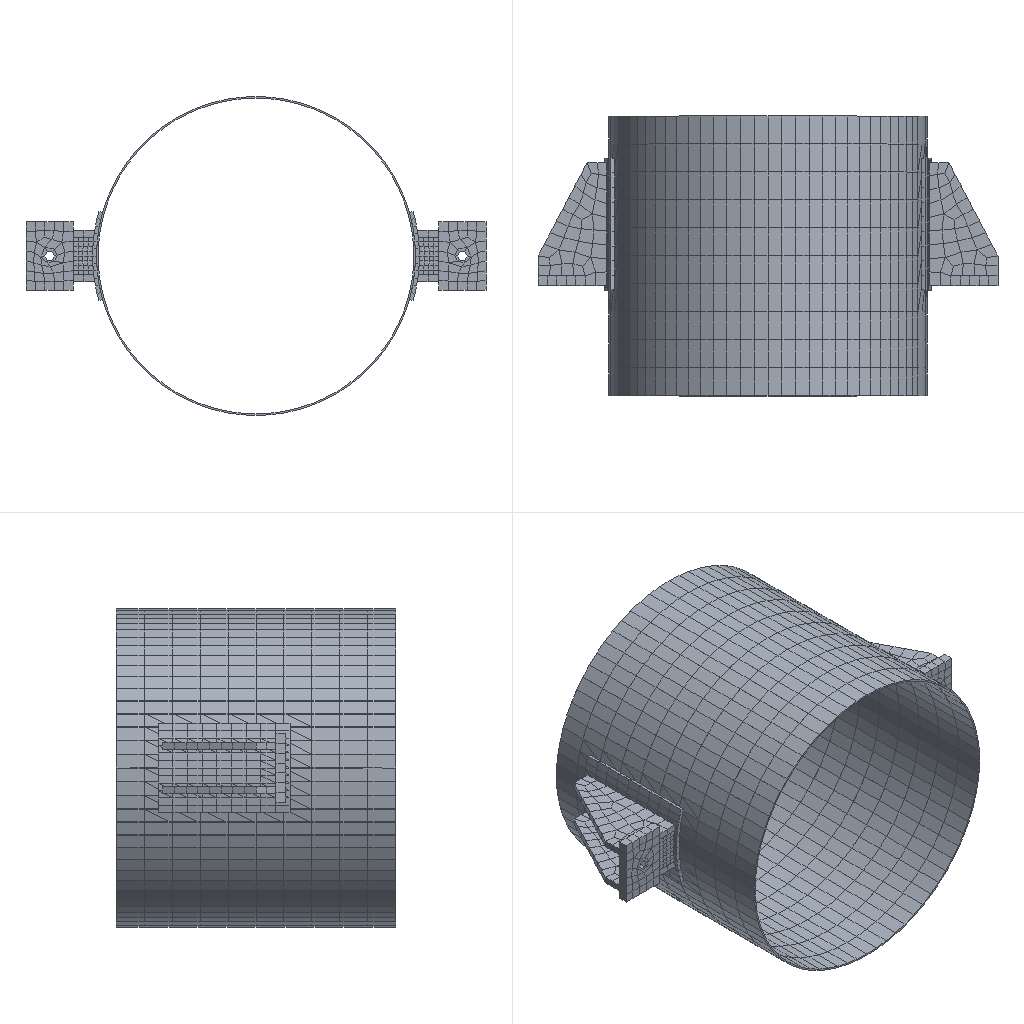Simulation study | ansys workbench
Ansys APDL input file, long lists of numbers shortened:
/batch
/config,noeldb,1     ! force off writing results to database
*get,_wallstrt,active,,time,wall
! ANSYS input file written by Workbench version 2022 R1
! File used for geometry attach:
/title,wbnew--____ (B5)
! ****** Begin Custom Load Command Snippet ******
/COM, ACT Extensions:
/COM,     LSDYNA, 2021.1
/COM,
! ****** End   Custom Load Command Snippet ******
*DIM,_wb_ProjectScratch_dir,string,248
_wb_ProjectScratch_dir(1) = ''
*DIM,_wb_SolverFiles_dir,string,248
_wb_SolverFiles_dir(1) = ''
*DIM,_wb_userfiles_dir,string,248
_wb_userfiles_dir(1) = ''
/com,--- Data in consistent NMM units. See Solving Units in the help system for more information.
/units,MPA
/nopr
/wb,file,start              !  signify a WB generated input file
/prep7
! Turn off shape checking because checks already performed inside WB mesher.
! See help system for more information.
SHPP,OFF,,NOWARN
/nolist
etcon,set             ! allow ANSYS to choose best KEYOP's for 180x elements, resets any applicable keyopt to MAPDL defaults
/com,*********** Nodes for the whole assembly ***********
nblock,3,,11156
(1i9,3e20.9e3)
        1    -9.929159159E+02     6.715040761E+02    -9.500000000E+01
! (10141 more lines like these left out)
-1
/wb,elem,start            !  set before creation of elements
/com,*********** Elements for Body 1 "__1^___1|__-__1" ***********
et,1,186
keyo,1,2,1          ! set full integration on SOLID186
eblock,19,solid,,720
(19i9)
        1        1        1        1        0        0        0        0       20        0      583     5200     5908     5907     5201     5204     5943     5942     5202
! (1439 more lines like these left out)
-1
/com,*********** Elements for Body 2 "__2^___1|__-__1" ***********
et,2,186
keyo,2,2,1          ! set full integration on SOLID186
eblock,19,solid,,108
(19i9)
        2        2        2        2        0        0        0        0       20        0      394     3257     3307     3371     3379     3293     3294     3370     3423
! (215 more lines like these left out)
-1
/com,*********** Elements for Body 3 "__3^___1|__-__1" ***********
et,3,186
keyo,3,2,1          ! set full integration on SOLID186
eblock,19,solid,,43
(19i9)
        3        3        3        3        0        0        0        0       20        0      103      797      820      801      798      844      821      840      843
! (85 more lines like these left out)
-1
/com,*********** Elements for Body 4 "__4^___1|__-__1" ***********
et,4,186
keyo,4,2,1          ! set full integration on SOLID186
eblock,19,solid,,38
(19i9)
        4        4        4        4        0        0        0        0       20        0      210     1631     1642     1646     1636     1662     1651     1647     1657
! (75 more lines like these left out)
-1
/com,*********** Elements for Body 5 "__4^___1|__-__1[2]" ***********
et,5,186
keyo,5,2,1          ! set full integration on SOLID186
eblock,19,solid,,38
(19i9)
        5        5        5        5        0        0        0        0       20        0      356     2834     2845     2849     2839     2865     2854     2850     2860
! (75 more lines like these left out)
-1
! (6 more sections like these left out)
/wb,elem,end               !  done creating elements
/com,*********** Send User Defined Coordinate System(s) ***********
csys,0
toffst,273.15,  ! Temperature offset from absolute zero
/com,*********** Set Reference Temperature ***********
tref,22.
/wb,mat,start              !  starting to send materials
/com,*********** Send Materials ***********
Temperature = 'TEMP' ! Temperature
MP,DENS,1,7.85e-09,	! tonne mm^-3
MP,ALPX,1,1.2e-05,	! C^-1
MP,C,1,434000000,	! mm^2 s^-2 C^-1
MP,KXX,1,60.5,	! tonne mm s^-3 C^-1
MP,RSVX,1,0.00017,	! ohm mm
MP,EX,1,200000,	! tonne s^-2 mm^-1
MP,NUXY,1,0.3,
MP,MURX,1,10000,
Temperature = 'TEMP' ! Temperature
MP,DENS,2,7.85e-09,	! tonne mm^-3
MP,ALPX,2,1.2e-05,	! C^-1
MP,C,2,434000000,	! mm^2 s^-2 C^-1
MP,KXX,2,60.5,	! tonne mm s^-3 C^-1
MP,RSVX,2,0.00017,	! ohm mm
MP,EX,2,200000,	! tonne s^-2 mm^-1
MP,NUXY,2,0.3,
MP,MURX,2,10000,
Temperature = 'TEMP' ! Temperature
MP,DENS,3,7.85e-09,	! tonne mm^-3
MP,ALPX,3,1.2e-05,	! C^-1
MP,C,3,434000000,	! mm^2 s^-2 C^-1
MP,KXX,3,60.5,	! tonne mm s^-3 C^-1
MP,RSVX,3,0.00017,	! ohm mm
MP,EX,3,200000,	! tonne s^-2 mm^-1
MP,NUXY,3,0.3,
MP,MURX,3,10000,
Temperature = 'TEMP' ! Temperature
MP,DENS,4,7.85e-09,	! tonne mm^-3
MP,ALPX,4,1.2e-05,	! C^-1
MP,C,4,434000000,	! mm^2 s^-2 C^-1
MP,KXX,4,60.5,	! tonne mm s^-3 C^-1
MP,RSVX,4,0.00017,	! ohm mm
MP,EX,4,200000,	! tonne s^-2 mm^-1
MP,NUXY,4,0.3,
MP,MURX,4,10000,
Temperature = 'TEMP' ! Temperature
MP,DENS,5,7.85e-09,	! tonne mm^-3
MP,ALPX,5,1.2e-05,	! C^-1
MP,C,5,434000000,	! mm^2 s^-2 C^-1
MP,KXX,5,60.5,	! tonne mm s^-3 C^-1
MP,RSVX,5,0.00017,	! ohm mm
MP,EX,5,200000,	! tonne s^-2 mm^-1
MP,NUXY,5,0.3,
MP,MURX,5,10000,
Temperature = 'TEMP' ! Temperature
MP,DENS,6,7.85e-09,	! tonne mm^-3
MP,ALPX,6,1.2e-05,	! C^-1
MP,C,6,434000000,	! mm^2 s^-2 C^-1
MP,KXX,6,60.5,	! tonne mm s^-3 C^-1
MP,RSVX,6,0.00017,	! ohm mm
MP,EX,6,200000,	! tonne s^-2 mm^-1
MP,NUXY,6,0.3,
MP,MURX,6,10000,
Temperature = 'TEMP' ! Temperature
MP,DENS,7,7.85e-09,	! tonne mm^-3
MP,ALPX,7,1.2e-05,	! C^-1
MP,C,7,434000000,	! mm^2 s^-2 C^-1
MP,KXX,7,60.5,	! tonne mm s^-3 C^-1
MP,RSVX,7,0.00017,	! ohm mm
MP,EX,7,200000,	! tonne s^-2 mm^-1
MP,NUXY,7,0.3,
MP,MURX,7,10000,
Temperature = 'TEMP' ! Temperature
MP,DENS,8,7.85e-09,	! tonne mm^-3
MP,ALPX,8,1.2e-05,	! C^-1
MP,C,8,434000000,	! mm^2 s^-2 C^-1
MP,KXX,8,60.5,	! tonne mm s^-3 C^-1
MP,RSVX,8,0.00017,	! ohm mm
MP,EX,8,200000,	! tonne s^-2 mm^-1
MP,NUXY,8,0.3,
MP,MURX,8,10000,
Temperature = 'TEMP' ! Temperature
MP,DENS,9,7.85e-09,	! tonne mm^-3
MP,ALPX,9,1.2e-05,	! C^-1
MP,C,9,434000000,	! mm^2 s^-2 C^-1
MP,KXX,9,60.5,	! tonne mm s^-3 C^-1
MP,RSVX,9,0.00017,	! ohm mm
MP,EX,9,200000,	! tonne s^-2 mm^-1
MP,NUXY,9,0.3,
MP,MURX,9,10000,
Temperature = 'TEMP' ! Temperature
MP,DENS,10,7.85e-09,	! tonne mm^-3
MP,ALPX,10,1.2e-05,	! C^-1
MP,C,10,434000000,	! mm^2 s^-2 C^-1
MP,KXX,10,60.5,	! tonne mm s^-3 C^-1
MP,RSVX,10,0.00017,	! ohm mm
MP,EX,10,200000,	! tonne s^-2 mm^-1
MP,NUXY,10,0.3,
MP,MURX,10,10000,
Temperature = 'TEMP' ! Temperature
MP,DENS,11,7.85e-09,	! tonne mm^-3
MP,ALPX,11,1.2e-05,	! C^-1
MP,C,11,434000000,	! mm^2 s^-2 C^-1
MP,KXX,11,60.5,	! tonne mm s^-3 C^-1
MP,RSVX,11,0.00017,	! ohm mm
MP,EX,11,200000,	! tonne s^-2 mm^-1
MP,NUXY,11,0.3,
MP,MURX,11,10000,
/wb,mat,end                !  done sending materials
!************************* Model Summary ********************
!__1^___1|__-__1,	结构钢,	matid,	1
!__2^___1|__-__1,	结构钢,	matid,	2
!__3^___1|__-__1,	结构钢,	matid,	3
!__4^___1|__-__1,	结构钢,	matid,	4
!__4^___1|__-__1[2],	结构钢,	matid,	5
!__5^___1|__-__1,	结构钢,	matid,	6
!__2^___1|__-__1[2],	结构钢,	matid,	7
!__4^___1|__-__1[3],	结构钢,	matid,	8
!__4^___1|__-__1[4],	结构钢,	matid,	9
!__3^___1|__-__1[2],	结构钢,	matid,	10
!__5^___1|__-__1[2],	结构钢,	matid,	11
!************************* End Model Summary ********************
! get the diagonal of the bounding box. Needed later for other things
*get,_xmin,node,,mnloc,x
*get,_ymin,node,,mnloc,y
*get,_zmin,node,,mnloc,z
*get,_xmax,node,,mxloc,x
*get,_ymax,node,,mxloc,y
*get,_zmax,node,,mxloc,z
_ASMDIAG=(_xmax-_xmin)*(_xmax-_xmin)+(_ymax-_ymin)*(_ymax-_ymin)+(_zmax-_zmin)*(_zmax-_zmin)
_ASMDIAG=SQRT(_ASMDIAG)
/wb,contact,start          !  starting to send contact
/com,*********** Create Contact "接触区域" ***********
/com,            Real Constant Set For Above Contact Is 13 & 12
*set,tid,13
*set,cid,12
r,tid
r,cid
et,tid,170
et,cid,174
eblock,10,,,48
(15i9)
     4275       13       13       13        0     5305     5306     5271     5270     7916     7814     7810     7811
! (47 more lines like these left out)
-1
eblock,10,,,48
(15i9)
     4323       12       12       12        0     5305     5306     5271     5270     7916     7814     7810     7811
! (47 more lines like these left out)
-1
eblock,10,,,108
(15i9)
     4371       12       13       12        0     3308     3253     3298     3299     3672     3671     3808     3810
! (107 more lines like these left out)
-1
eblock,10,,,108
(15i9)
     4479       13       12       13        0     3308     3253     3298     3299     3672     3671     3808     3810
! (107 more lines like these left out)
-1
keyo,cid,8,2               ! auto create asymmetric contact (from Program Controlled setting)
keyo,cid,10,0              ! adjust contact stiffness each NR iteration (from Program Controlled setting)
keyo,cid,12,5              ! bonded always
keyo,cid,18,1              ! small sliding turned on by application
keyo,cid,2,0               ! augmented Lagrange (from Program Controlled setting)
keyo,cid,4,0               ! on Gauss point (from Program Controlled setting)
keyo,cid,9,1               ! ignore initial gaps/penetration
keyo,cid,7,0               ! No Prediction
rmod,tid,3,10.      ! FKN
rmod,tid,5,0.       ! ICONT
rmod,tid,6,0.       ! PINB
rmod,tid,10,0.      ! CNOF
rmod,tid,12,0.      ! FKT
rmod,tid,36,56      ! WB DSID
rmod,cid,3,10.      ! FKN
rmod,cid,5,0.       ! ICONT
rmod,cid,6,0.       ! PINB
rmod,cid,10,0.      ! CNOF
rmod,cid,12,0.      ! FKT
rmod,cid,36,56      ! WB DSID
/com,*********** Create Contact "接触区域 2" ***********
/com,            Real Constant Set For Above Contact Is 15 & 14
*set,tid,15
*set,cid,14
r,tid
r,cid
et,tid,170
et,cid,174
eblock,10,,,48
(15i9)
     4587       15       15       15        0     5675     5676     5641     5640     8928     8862     8859     8860
! (47 more lines like these left out)
-1
eblock,10,,,48
(15i9)
     4635       14       14       14        0     5675     5676     5641     5640     8928     8862     8859     8860
! (47 more lines like these left out)
-1
eblock,10,,,108
(15i9)
     4683       14       15       14        0     2105     2050     2095     2096     2469     2468     2605     2607
! (107 more lines like these left out)
-1
eblock,10,,,108
(15i9)
     4791       15       14       15        0     2105     2050     2095     2096     2469     2468     2605     2607
! (107 more lines like these left out)
-1
keyo,cid,8,2               ! auto create asymmetric contact (from Program Controlled setting)
keyo,cid,10,0              ! adjust contact stiffness each NR iteration (from Program Controlled setting)
keyo,cid,12,5              ! bonded always
keyo,cid,18,1              ! small sliding turned on by application
keyo,cid,2,0               ! augmented Lagrange (from Program Controlled setting)
keyo,cid,4,0               ! on Gauss point (from Program Controlled setting)
keyo,cid,9,1               ! ignore initial gaps/penetration
keyo,cid,7,0               ! No Prediction
rmod,tid,3,10.      ! FKN
rmod,tid,5,0.       ! ICONT
rmod,tid,6,0.       ! PINB
rmod,tid,10,0.      ! CNOF
rmod,tid,12,0.      ! FKT
rmod,tid,36,59      ! WB DSID
rmod,cid,3,10.      ! FKN
rmod,cid,5,0.       ! ICONT
rmod,cid,6,0.       ! PINB
rmod,cid,10,0.      ! CNOF
rmod,cid,12,0.      ! FKT
rmod,cid,36,59      ! WB DSID
/com,*********** Create Contact "接触区域 3" ***********
/com,            Real Constant Set For Above Contact Is 17 & 16
*set,tid,17
*set,cid,16
r,tid
r,cid
et,tid,170
et,cid,174
eblock,10,,,18
(15i9)
     4899       17       17       17        0     3191     3192     3233     3234     3492     3498     3622     3494
! (17 more lines like these left out)
-1
eblock,10,,,18
(15i9)
     4917       16       16       16        0     3191     3192     3233     3234     3492     3498     3622     3494
! (17 more lines like these left out)
-1
eblock,10,,,9
(15i9)
     4935       16       17       16        0     1719     1720     1679     1680     1953     1893     1892     1895
! (8 more lines like these left out)
-1
eblock,10,,,9
(15i9)
     4944       17       16       17        0     1719     1720     1679     1680     1953     1893     1892     1895
! (8 more lines like these left out)
-1
keyo,cid,8,2               ! auto create asymmetric contact (from Program Controlled setting)
keyo,cid,10,0              ! adjust contact stiffness each NR iteration (from Program Controlled setting)
keyo,cid,12,5              ! bonded always
keyo,cid,18,1              ! small sliding turned on by application
keyo,cid,2,0               ! augmented Lagrange (from Program Controlled setting)
keyo,cid,4,0               ! on Gauss point (from Program Controlled setting)
keyo,cid,9,1               ! ignore initial gaps/penetration
keyo,cid,7,0               ! No Prediction
rmod,tid,3,10.      ! FKN
rmod,tid,5,0.       ! ICONT
rmod,tid,6,0.       ! PINB
rmod,tid,10,0.      ! CNOF
rmod,tid,12,0.      ! FKT
rmod,tid,36,62      ! WB DSID
rmod,cid,3,10.      ! FKN
rmod,cid,5,0.       ! ICONT
rmod,cid,6,0.       ! PINB
rmod,cid,10,0.      ! CNOF
rmod,cid,12,0.      ! FKT
rmod,cid,36,62      ! WB DSID
/com,*********** Create Contact "接触区域 4" ***********
/com,            Real Constant Set For Above Contact Is 19 & 18
*set,tid,19
*set,cid,18
r,tid
r,cid
et,tid,170
et,cid,174
eblock,10,,,18
(15i9)
     4953       19       19       19        0     3380     3381     3421     3422     3955     3960     4026     3957
! (17 more lines like these left out)
-1
eblock,10,,,18
(15i9)
     4971       18       18       18        0     3380     3381     3421     3422     3955     3960     4026     3957
! (17 more lines like these left out)
-1
eblock,10,,,9
(15i9)
     4989       18       19       18        0     2922     2923     2882     2883     3156     3096     3095     3098
! (8 more lines like these left out)
-1
eblock,10,,,9
(15i9)
     4998       19       18       19        0     2922     2923     2882     2883     3156     3096     3095     3098
! (8 more lines like these left out)
-1
keyo,cid,8,2               ! auto create asymmetric contact (from Program Controlled setting)
keyo,cid,10,0              ! adjust contact stiffness each NR iteration (from Program Controlled setting)
keyo,cid,12,5              ! bonded always
keyo,cid,18,1              ! small sliding turned on by application
keyo,cid,2,0               ! augmented Lagrange (from Program Controlled setting)
keyo,cid,4,0               ! on Gauss point (from Program Controlled setting)
keyo,cid,9,1               ! ignore initial gaps/penetration
keyo,cid,7,0               ! No Prediction
rmod,tid,3,10.      ! FKN
rmod,tid,5,0.       ! ICONT
rmod,tid,6,0.       ! PINB
rmod,tid,10,0.      ! CNOF
rmod,tid,12,0.      ! FKT
rmod,tid,36,65      ! WB DSID
rmod,cid,3,10.      ! FKN
rmod,cid,5,0.       ! ICONT
rmod,cid,6,0.       ! PINB
rmod,cid,10,0.      ! CNOF
rmod,cid,12,0.      ! FKT
rmod,cid,36,65      ! WB DSID
/com,*********** Create Contact "接触区域 5" ***********
/com,            Real Constant Set For Above Contact Is 21 & 20
*set,tid,21
*set,cid,20
r,tid
r,cid
et,tid,170
et,cid,174
eblock,10,,,12
(15i9)
     5007       21       21       21        0     3245     3190     3235     3236     3490     3489     3626     3628
! (11 more lines like these left out)
-1
eblock,10,,,12
(15i9)
     5019       20       20       20        0     3245     3190     3235     3236     3490     3489     3626     3628
! (11 more lines like these left out)
-1
eblock,10,,,16
(15i9)
     5031       20       21       20        0     1273     1298     1234     1250     1580     1508     1507     1540
! (15 more lines like these left out)
-1
eblock,10,,,16
(15i9)
     5047       21       20       21        0     1273     1298     1234     1250     1580     1508     1507     1540
! (15 more lines like these left out)
-1
keyo,cid,8,2               ! auto create asymmetric contact (from Program Controlled setting)
keyo,cid,10,0              ! adjust contact stiffness each NR iteration (from Program Controlled setting)
keyo,cid,12,5              ! bonded always
keyo,cid,18,1              ! small sliding turned on by application
keyo,cid,2,0               ! augmented Lagrange (from Program Controlled setting)
keyo,cid,4,0               ! on Gauss point (from Program Controlled setting)
keyo,cid,9,1               ! ignore initial gaps/penetration
keyo,cid,7,0               ! No Prediction
rmod,tid,3,10.      ! FKN
rmod,tid,5,0.       ! ICONT
rmod,tid,6,0.       ! PINB
rmod,tid,10,0.      ! CNOF
rmod,tid,12,0.      ! FKT
rmod,tid,36,68      ! WB DSID
rmod,cid,3,10.      ! FKN
rmod,cid,5,0.       ! ICONT
rmod,cid,6,0.       ! PINB
rmod,cid,10,0.      ! CNOF
rmod,cid,12,0.      ! FKT
rmod,cid,36,68      ! WB DSID
! (13 more sections like these left out)
/wb,contact,end            !  done creating contacts
/golist
/wb,load,start             !  starting to send loads
/com,*********** Fixed Supports ***********
CMBLOCK,_FIXEDSU,NODE,       60
(8i10)
       849       850       875       876       877       878       879       880
! (7 more lines like these left out)
cmsel,s,_FIXEDSU
d,all,all
nsel,all
/com,*********** Define Force Using Surface Effect Elements ***********
local,12,0,0.,0.,0.,0.,0.,0.
csys,0
et,48,154
eblock,10,,,86
(15i9)
     5571       48       48       48       12     4075     4078     4079     4056     4297     4302     4246     4244
! (85 more lines like these left out)
-1
esel,s,type,,48
keyop,48,2,1                ! Apply load in local coordinate system
keyop,48,7,1                ! Use original area so load is constant in large deformation
esel,all
/gst,on,on
fini
*get,_numnode,node,0,count
*get,_numelem,elem,0,count
*get, _MAXELEMNUM, elem, 0, NUM, MAX
*get, _MAXNODENUM, node, 0, NUM, MAX
*get, _MAXELEMTYPE, etyp, 0, NUM, MAX
*get, _MAXREALCONST, real, 0, NUM, MAX
/go
/wb,load,end               !  done creating loads
/com,--- Number of total nodes = %_numnode%
/com,--- Number of contact elements = 1382
/com,--- Number of spring elements = 0
/com,--- Number of bearing elements = 0
/com,--- Number of solid elements = 1302
/com,--- Number of condensed parts = 0
/com,--- Number of total elements = %_numelem%
*get,_wallbsol,active,,time,wall
/com,****************************************************************************
/com,*************************    SOLUTION       ********************************
/com,****************************************************************************
/solu
antype,0                   ! static analysis
_thickRatio=  0     ! Ratio of thick parts in the model
eqsl,sparse,,,,,1
cntr,print,1               ! print out contact info and also make no initial contact an error
dmpoption,emat,no             ! Don't combine emat file for DANSYS
dmpoption,esav,no             ! Don't combine esav file for DANSYS
nldiag,cont,iter           ! print out contact info each equilibrium iteration
rescontrol,,none                 ! Do not keep any restart files
/com,****************************************************
/com,******************* SOLVE FOR LS 1 OF 1 ****************
esel,s,type,,48
nsle
sfe,all,1,pres,1,0.
sfe,all,2,pres,1,0.9125
sfe,all,3,pres,1,0.
nsel,all
esel,all
/nopr
/gopr
nsub,1,1,1
time,1.
outres,erase
outres,all,none
outres,nsol,all,
outres,rsol,all
outres,eangl,all
outres,etmp,all
outres,veng,all
outres,strs,all,
outres,epel,all,
outres,eppl,all,
outres,cont,all,
! *********** WB SOLVE COMMAND ***********
! check interactive state
*get,ANSINTER_,active,,int
*if,ANSINTER_,ne,0,then
/eof
*endif
solve
/com *************** Write FE CONNECTORS *********
CEWRITE,file,ce,,INTE
/com,****************************************************
/com,*************** FINISHED SOLVE FOR LS 1 *************
*get,_wallasol,active,,time,wall
/nopr
*get,_numnode,node,0,count
*get,_numelem,elem,0,count
*get, _MAXELEMNUM, elem, 0, NUM, MAX
*get, _MAXNODENUM, node, 0, NUM, MAX,,,INTERNAL
*get, _MAXELEMTYPE, etyp, 0, NUM, MAX
*get, _MAXREALCONST, real, 0, NUM, MAX
/gopr
/post1
xmlo,ENCODING,ISO-8859-1
xmlo,parm
/xml,parm,xml
fini
/gopr
*get,_walldone,active,,time,wall
_preptime=(_wallbsol-_wallstrt)*3600
_solvtime=(_wallasol-_wallbsol)*3600
_posttime=(_walldone-_wallasol)*3600
_totaltim=(_walldone-_wallstrt)*3600
*get,_dlbratio,active,0,solu,dlbr
*get,_combtime,active,0,solu,comb
*get,_ssmode,active,0,solu,ssmm
*get,_ndofs,active,0,solu,ndof
*get,_sol_end_time,active,0,set,time
*if,_sol_end_time,eq,1.,then
/fclean				!clean distributed files
*endif
/com,--- Total number of nodes = %_numnode%
/com,--- Total number of elements = %_numelem%
/com,--- Element load balance ratio = %_dlbratio%
/com,--- Time to combine distributed files = %_combtime%
/com,--- Sparse memory mode = %_ssmode%
/com,--- Number of DOF = %_ndofs%
/wb,file,end               ! done with WB generated input